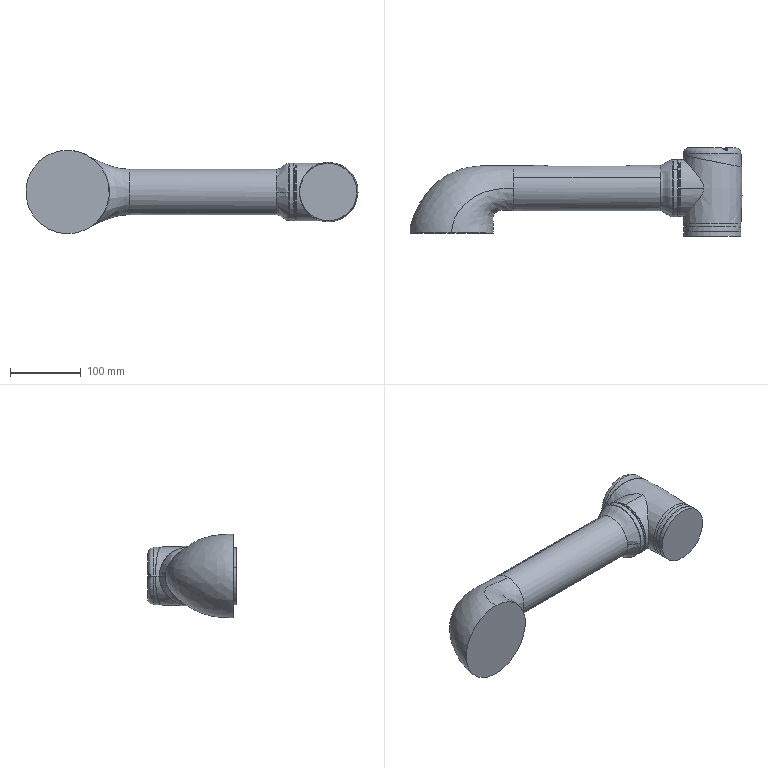Part | SolidWorks | features BaseBody 3, Fillet 1, ICE 1, RefAxis 1, RefPoint 1 | 3 solids | 379 faces | box 469.687 x 125 x 118 mm | volume 2299824 mm3 | plane 262 | spline 80 | cylinder 27 | torus 10 | commonest cylinder face diameters 81 x14 8 x7 50 x2 64 x2 79.988 x2